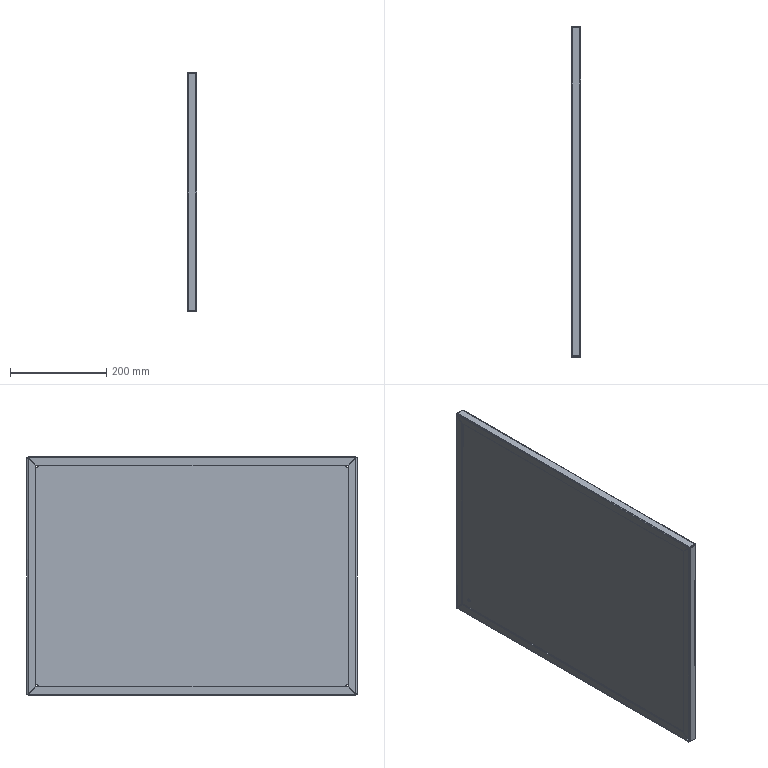Part | STEP file | PN_0076 front door | 1 solid | 78 faces | box 20 x 687 x 497 mm | volume 627548 mm3 | plane 38 | cylinder 24 | spline 16 | commonest cylinder face diameters 1.473 x8 4.473 x8 6 x8